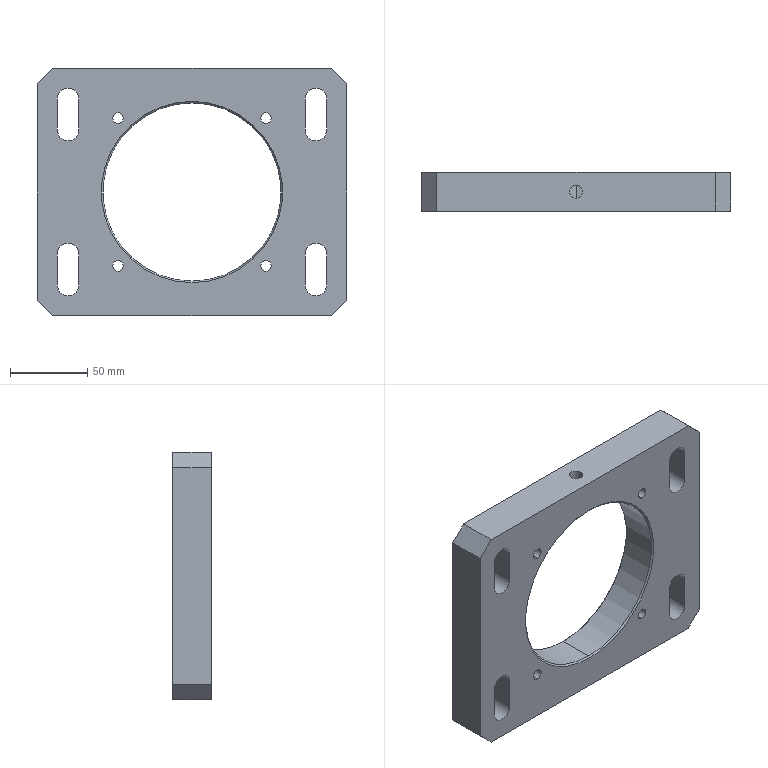Part | STEP file | HXGR200008-05-12-01 | 1 solid | 46 faces | box 200 x 25 x 160 mm | volume 486660 mm3 | cylinder 24 | plane 18 | cone 4 | commonest cylinder face diameters 14 x12 6.8 x8 8.5 x2 115 x2